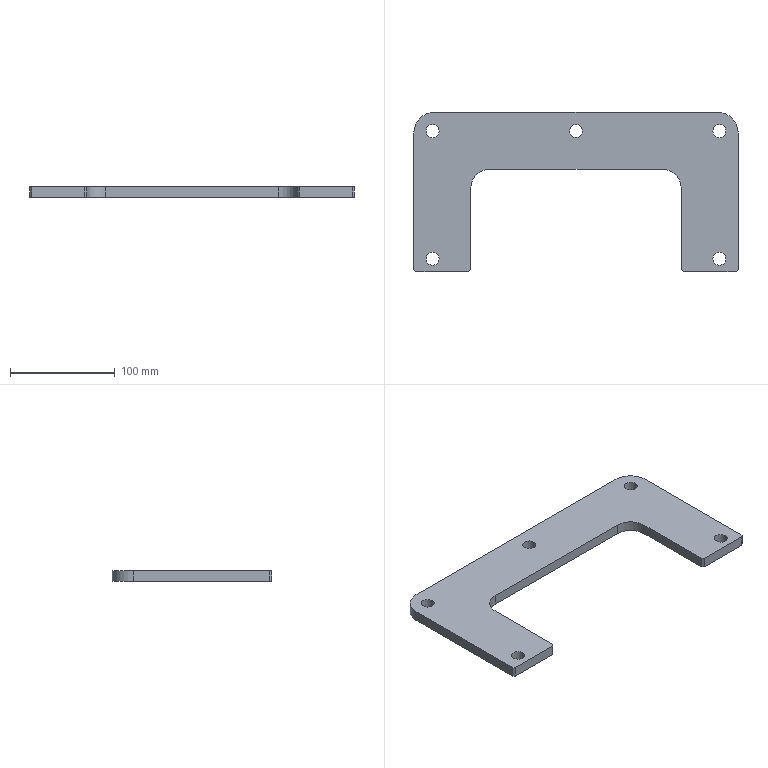Part | SolidWorks | features Chamfer 1, Extrusion 1, ICE 1 | 1 solid | 28 faces | box 310 x 152.5 x 10 mm | volume 269228 mm3 | cylinder 14 | plane 14 | commonest cylinder face diameters 12.5 x10 36 x2 40 x2
STEP:
#1=CARTESIAN_POINT('',(-143.25,15.,0.));
#2=VERTEX_POINT('',#1);
#3=CARTESIAN_POINT('',(-130.75,15.,0.));
#4=VERTEX_POINT('',#3);
#5=CARTESIAN_POINT('',(-137.,15.,0.));
#6=DIRECTION('',(0.,0.,1.));
#7=DIRECTION('',(1.,0.,0.));
#8=AXIS2_PLACEMENT_3D('',#5,#6,#7);
#9=CIRCLE('',#8,6.25);
#10=EDGE_CURVE('',#2,#4,#9,.T.);
#11=ORIENTED_EDGE('',*,*,#10,.F.);
#12=CARTESIAN_POINT('',(-143.25,15.,10.));
#13=VERTEX_POINT('',#12);
#14=CARTESIAN_POINT('',(-143.25,15.,0.));
#15=DIRECTION('',(0.,0.,1.));
#16=VECTOR('',#15,1000.);
#17=LINE('',#14,#16);
#18=EDGE_CURVE('',#2,#13,#17,.T.);
#19=ORIENTED_EDGE('',*,*,#18,.T.);
#20=CARTESIAN_POINT('',(-130.75,15.,10.));
#21=VERTEX_POINT('',#20);
#22=CARTESIAN_POINT('',(-137.,15.,10.));
#23=DIRECTION('',(0.,0.,1.));
#24=DIRECTION('',(1.,0.,0.));
#25=AXIS2_PLACEMENT_3D('',#22,#23,#24);
#26=CIRCLE('',#25,6.25);
#27=EDGE_CURVE('',#13,#21,#26,.T.);
#28=ORIENTED_EDGE('',*,*,#27,.T.);
#29=CARTESIAN_POINT('',(-130.75,15.,0.));
#30=DIRECTION('',(0.,0.,1.));
#31=VECTOR('',#30,1000.);
#32=LINE('',#29,#31);
#33=EDGE_CURVE('',#4,#21,#32,.T.);
#34=ORIENTED_EDGE('',*,*,#33,.F.);
#35=EDGE_LOOP('',(#11,#19,#28,#34));
#36=FACE_OUTER_BOUND('',#35,.T.);
#37=CARTESIAN_POINT('',(-137.,15.,0.));
#38=DIRECTION('',(0.,0.,1.));
#39=DIRECTION('',(1.,0.,0.));
#40=AXIS2_PLACEMENT_3D('',#37,#38,#39);
#41=CYLINDRICAL_SURFACE('',#40,6.25);
#42=ADVANCED_FACE('',(#36),#41,.F.);
#43=CARTESIAN_POINT('',(130.75,15.,0.));
#44=VERTEX_POINT('',#43);
#45=CARTESIAN_POINT('',(143.25,15.,0.));
#46=VERTEX_POINT('',#45);
#47=CARTESIAN_POINT('',(137.,15.,0.));
#48=DIRECTION('',(0.,0.,1.));
#49=DIRECTION('',(-1.,0.,0.));
#50=AXIS2_PLACEMENT_3D('',#47,#48,#49);
#51=CIRCLE('',#50,6.25);
#52=EDGE_CURVE('',#44,#46,#51,.T.);
#53=ORIENTED_EDGE('',*,*,#52,.F.);
#54=CARTESIAN_POINT('',(130.75,15.,10.));
#55=VERTEX_POINT('',#54);
#56=CARTESIAN_POINT('',(130.75,15.,0.));
#57=DIRECTION('',(0.,0.,1.));
#58=VECTOR('',#57,1000.);
#59=LINE('',#56,#58);
#60=EDGE_CURVE('',#44,#55,#59,.T.);
#61=ORIENTED_EDGE('',*,*,#60,.T.);
#62=CARTESIAN_POINT('',(143.25,15.,10.));
#63=VERTEX_POINT('',#62);
#64=CARTESIAN_POINT('',(137.,15.,10.));
#65=DIRECTION('',(0.,0.,1.));
#66=DIRECTION('',(-1.,0.,0.));
#67=AXIS2_PLACEMENT_3D('',#64,#65,#66);
#68=CIRCLE('',#67,6.25);
#69=EDGE_CURVE('',#55,#63,#68,.T.);
#70=ORIENTED_EDGE('',*,*,#69,.T.);
#71=CARTESIAN_POINT('',(143.25,15.,0.));
#72=DIRECTION('',(0.,0.,1.));
#73=VECTOR('',#72,1000.);
#74=LINE('',#71,#73);
#75=EDGE_CURVE('',#46,#63,#74,.T.);
#76=ORIENTED_EDGE('',*,*,#75,.F.);
#77=EDGE_LOOP('',(#53,#61,#70,#76));
#78=FACE_OUTER_BOUND('',#77,.T.);
#79=CARTESIAN_POINT('',(137.,15.,0.));
#80=DIRECTION('',(0.,0.,1.));
#81=DIRECTION('',(1.,0.,0.));
#82=AXIS2_PLACEMENT_3D('',#79,#80,#81);
#83=CYLINDRICAL_SURFACE('',#82,6.25);
#84=ADVANCED_FACE('',(#78),#83,.F.);
#85=CARTESIAN_POINT('',(-143.25,137.,0.));
#86=VERTEX_POINT('',#85);
#87=CARTESIAN_POINT('',(-130.75,137.,0.));
#88=VERTEX_POINT('',#87);
#89=CARTESIAN_POINT('',(-137.,137.,0.));
#90=DIRECTION('',(0.,0.,1.));
#91=DIRECTION('',(1.,0.,0.));
#92=AXIS2_PLACEMENT_3D('',#89,#90,#91);
#93=CIRCLE('',#92,6.25);
#94=EDGE_CURVE('',#86,#88,#93,.T.);
#95=ORIENTED_EDGE('',*,*,#94,.F.);
#96=CARTESIAN_POINT('',(-143.25,137.,10.));
#97=VERTEX_POINT('',#96);
#98=CARTESIAN_POINT('',(-143.25,137.,0.));
#99=DIRECTION('',(0.,0.,1.));
#100=VECTOR('',#99,1000.);
#101=LINE('',#98,#100);
#102=EDGE_CURVE('',#86,#97,#101,.T.);
#103=ORIENTED_EDGE('',*,*,#102,.T.);
#104=CARTESIAN_POINT('',(-130.75,137.,10.));
#105=VERTEX_POINT('',#104);
#106=CARTESIAN_POINT('',(-137.,137.,10.));
#107=DIRECTION('',(0.,0.,1.));
#108=DIRECTION('',(1.,0.,0.));
#109=AXIS2_PLACEMENT_3D('',#106,#107,#108);
#110=CIRCLE('',#109,6.25);
#111=EDGE_CURVE('',#97,#105,#110,.T.);
#112=ORIENTED_EDGE('',*,*,#111,.T.);
#113=CARTESIAN_POINT('',(-130.75,137.,0.));
#114=DIRECTION('',(0.,0.,1.));
#115=VECTOR('',#114,1000.);
#116=LINE('',#113,#115);
#117=EDGE_CURVE('',#88,#105,#116,.T.);
#118=ORIENTED_EDGE('',*,*,#117,.F.);
#119=EDGE_LOOP('',(#95,#103,#112,#118));
#120=FACE_OUTER_BOUND('',#119,.T.);
#121=CARTESIAN_POINT('',(-137.,137.,0.));
#122=DIRECTION('',(0.,0.,1.));
#123=DIRECTION('',(1.,0.,0.));
#124=AXIS2_PLACEMENT_3D('',#121,#122,#123);
#125=CYLINDRICAL_SURFACE('',#124,6.25);
#126=ADVANCED_FACE('',(#120),#125,.F.);
#127=CARTESIAN_POINT('',(130.75,137.,0.));
#128=VERTEX_POINT('',#127);
#129=CARTESIAN_POINT('',(143.25,137.,0.));
#130=VERTEX_POINT('',#129);
#131=CARTESIAN_POINT('',(137.,137.,0.));
#132=DIRECTION('',(0.,0.,1.));
#133=DIRECTION('',(1.,0.,0.));
#134=AXIS2_PLACEMENT_3D('',#131,#132,#133);
#135=CIRCLE('',#134,6.25);
#136=EDGE_CURVE('',#128,#130,#135,.T.);
#137=ORIENTED_EDGE('',*,*,#136,.F.);
#138=CARTESIAN_POINT('',(130.75,137.,10.));
#139=VERTEX_POINT('',#138);
#140=CARTESIAN_POINT('',(130.75,137.,0.));
#141=DIRECTION('',(0.,0.,1.));
#142=VECTOR('',#141,1000.);
#143=LINE('',#140,#142);
#144=EDGE_CURVE('',#128,#139,#143,.T.);
#145=ORIENTED_EDGE('',*,*,#144,.T.);
#146=CARTESIAN_POINT('',(143.25,137.,10.));
#147=VERTEX_POINT('',#146);
#148=CARTESIAN_POINT('',(137.,137.,10.));
#149=DIRECTION('',(0.,0.,1.));
#150=DIRECTION('',(1.,0.,0.));
#151=AXIS2_PLACEMENT_3D('',#148,#149,#150);
#152=CIRCLE('',#151,6.25);
#153=EDGE_CURVE('',#139,#147,#152,.T.);
#154=ORIENTED_EDGE('',*,*,#153,.T.);
#155=CARTESIAN_POINT('',(143.25,137.,0.));
#156=DIRECTION('',(0.,0.,1.));
#157=VECTOR('',#156,1000.);
#158=LINE('',#155,#157);
#159=EDGE_CURVE('',#130,#147,#158,.T.);
#160=ORIENTED_EDGE('',*,*,#159,.F.);
#161=EDGE_LOOP('',(#137,#145,#154,#160));
#162=FACE_OUTER_BOUND('',#161,.T.);
#163=CARTESIAN_POINT('',(137.,137.,0.));
#164=DIRECTION('',(0.,0.,1.));
#165=DIRECTION('',(1.,0.,0.));
#166=AXIS2_PLACEMENT_3D('',#163,#164,#165);
#167=CYLINDRICAL_SURFACE('',#166,6.25);
#168=ADVANCED_FACE('',(#162),#167,.F.);
#169=CARTESIAN_POINT('',(-6.25,137.,0.));
#170=VERTEX_POINT('',#169);
#171=CARTESIAN_POINT('',(6.25,137.,0.));
#172=VERTEX_POINT('',#171);
#173=CARTESIAN_POINT('',(0.,137.,0.));
#174=DIRECTION('',(0.,0.,1.));
#175=DIRECTION('',(1.,0.,0.));
#176=AXIS2_PLACEMENT_3D('',#173,#174,#175);
#177=CIRCLE('',#176,6.25);
#178=EDGE_CURVE('',#170,#172,#177,.T.);
#179=ORIENTED_EDGE('',*,*,#178,.F.);
#180=CARTESIAN_POINT('',(-6.25,137.,10.));
#181=VERTEX_POINT('',#180);
#182=CARTESIAN_POINT('',(-6.25,137.,0.));
#183=DIRECTION('',(0.,0.,1.));
#184=VECTOR('',#183,1000.);
#185=LINE('',#182,#184);
#186=EDGE_CURVE('',#170,#181,#185,.T.);
#187=ORIENTED_EDGE('',*,*,#186,.T.);
#188=CARTESIAN_POINT('',(6.25,137.,10.));
#189=VERTEX_POINT('',#188);
#190=CARTESIAN_POINT('',(0.,137.,10.));
#191=DIRECTION('',(0.,0.,1.));
#192=DIRECTION('',(1.,0.,0.));
#193=AXIS2_PLACEMENT_3D('',#190,#191,#192);
#194=CIRCLE('',#193,6.25);
#195=EDGE_CURVE('',#181,#189,#194,.T.);
#196=ORIENTED_EDGE('',*,*,#195,.T.);
#197=CARTESIAN_POINT('',(6.25,137.,0.));
#198=DIRECTION('',(0.,0.,1.));
#199=VECTOR('',#198,1000.);
#200=LINE('',#197,#199);
#201=EDGE_CURVE('',#172,#189,#200,.T.);
#202=ORIENTED_EDGE('',*,*,#201,.F.);
#203=EDGE_LOOP('',(#179,#187,#196,#202));
#204=FACE_OUTER_BOUND('',#203,.T.);
#205=CARTESIAN_POINT('',(0.,137.,0.));
#206=DIRECTION('',(0.,0.,1.));
#207=DIRECTION('',(1.,0.,0.));
#208=AXIS2_PLACEMENT_3D('',#205,#206,#207);
#209=CYLINDRICAL_SURFACE('',#208,6.25);
#210=ADVANCED_FACE('',(#204),#209,.F.);
#211=CARTESIAN_POINT('',(82.5,100.5,0.));
#212=VERTEX_POINT('',#211);
#213=CARTESIAN_POINT('',(100.5,82.5,0.));
#214=VERTEX_POINT('',#213);
#215=CARTESIAN_POINT('',(82.5,82.5,0.));
#216=DIRECTION('',(0.,0.,-1.));
#217=DIRECTION('',(1.,0.,0.));
#218=AXIS2_PLACEMENT_3D('',#215,#216,#217);
#219=CIRCLE('',#218,18.);
#220=EDGE_CURVE('',#212,#214,#219,.T.);
#221=ORIENTED_EDGE('',*,*,#220,.T.);
#222=CARTESIAN_POINT('',(100.5,82.5,10.));
#223=VERTEX_POINT('',#222);
#224=CARTESIAN_POINT('',(100.5,82.5,10.));
#225=DIRECTION('',(0.,0.,-1.));
#226=VECTOR('',#225,1000.);
#227=LINE('',#224,#226);
#228=EDGE_CURVE('',#223,#214,#227,.T.);
#229=ORIENTED_EDGE('',*,*,#228,.F.);
#230=CARTESIAN_POINT('',(82.5,100.5,10.));
#231=VERTEX_POINT('',#230);
#232=CARTESIAN_POINT('',(82.5,82.5,10.));
#233=DIRECTION('',(0.,0.,-1.));
#234=DIRECTION('',(1.,0.,0.));
#235=AXIS2_PLACEMENT_3D('',#232,#233,#234);
#236=CIRCLE('',#235,18.);
#237=EDGE_CURVE('',#231,#223,#236,.T.);
#238=ORIENTED_EDGE('',*,*,#237,.F.);
#239=CARTESIAN_POINT('',(82.5,100.5,10.));
#240=DIRECTION('',(0.,0.,-1.));
#241=VECTOR('',#240,1000.);
#242=LINE('',#239,#241);
#243=EDGE_CURVE('',#231,#212,#242,.T.);
#244=ORIENTED_EDGE('',*,*,#243,.T.);
#245=EDGE_LOOP('',(#221,#229,#238,#244));
#246=FACE_OUTER_BOUND('',#245,.T.);
#247=CARTESIAN_POINT('',(82.5,82.5,10.));
#248=DIRECTION('',(0.,0.,-1.));
#249=DIRECTION('',(-1.,0.,0.));
#250=AXIS2_PLACEMENT_3D('',#247,#248,#249);
#251=CYLINDRICAL_SURFACE('',#250,18.);
#252=ADVANCED_FACE('',(#246),#251,.F.);
#253=CARTESIAN_POINT('',(100.5,4.5,0.));
#254=VERTEX_POINT('',#253);
#255=CARTESIAN_POINT('',(100.5,82.5,0.));
#256=DIRECTION('',(0.,-1.,0.));
#257=VECTOR('',#256,1000.);
#258=LINE('',#255,#257);
#259=EDGE_CURVE('',#214,#254,#258,.T.);
#260=ORIENTED_EDGE('',*,*,#259,.T.);
#261=CARTESIAN_POINT('',(100.5,4.5,10.));
#262=VERTEX_POINT('',#261);
#263=CARTESIAN_POINT('',(100.5,4.5,10.));
#264=DIRECTION('',(0.,0.,1.));
#265=VECTOR('',#264,1000.);
#266=LINE('',#263,#265);
#267=EDGE_CURVE('',#254,#262,#266,.T.);
#268=ORIENTED_EDGE('',*,*,#267,.T.);
#269=CARTESIAN_POINT('',(100.5,82.5,10.));
#270=DIRECTION('',(0.,-1.,0.));
#271=VECTOR('',#270,1000.);
#272=LINE('',#269,#271);
#273=EDGE_CURVE('',#223,#262,#272,.T.);
#274=ORIENTED_EDGE('',*,*,#273,.F.);
#275=ORIENTED_EDGE('',*,*,#228,.T.);
#276=EDGE_LOOP('',(#260,#268,#274,#275));
#277=FACE_OUTER_BOUND('',#276,.T.);
#278=CARTESIAN_POINT('',(100.5,82.5,10.));
#279=DIRECTION('',(1.,0.,0.));
#280=DIRECTION('',(0.,0.,-1.));
#281=AXIS2_PLACEMENT_3D('',#278,#279,#280);
#282=PLANE('',#281);
#283=ADVANCED_FACE('',(#277),#282,.F.);
#284=CARTESIAN_POINT('',(102.5,2.5,0.));
#285=VERTEX_POINT('',#284);
#286=CARTESIAN_POINT('',(153.,2.5,0.));
#287=VERTEX_POINT('',#286);
#288=CARTESIAN_POINT('',(100.5,2.5,0.));
#289=DIRECTION('',(1.,0.,0.));
#290=VECTOR('',#289,1000.);
#291=LINE('',#288,#290);
#292=EDGE_CURVE('',#285,#287,#291,.T.);
#293=ORIENTED_EDGE('',*,*,#292,.T.);
#294=CARTESIAN_POINT('',(153.,2.5,10.));
#295=VERTEX_POINT('',#294);
#296=CARTESIAN_POINT('',(153.,2.5,10.));
#297=DIRECTION('',(0.,0.,1.));
#298=VECTOR('',#297,1000.);
#299=LINE('',#296,#298);
#300=EDGE_CURVE('',#287,#295,#299,.T.);
#301=ORIENTED_EDGE('',*,*,#300,.T.);
#302=CARTESIAN_POINT('',(102.5,2.5,10.));
#303=VERTEX_POINT('',#302);
#304=CARTESIAN_POINT('',(100.5,2.5,10.));
#305=DIRECTION('',(1.,0.,0.));
#306=VECTOR('',#305,1000.);
#307=LINE('',#304,#306);
#308=EDGE_CURVE('',#303,#295,#307,.T.);
#309=ORIENTED_EDGE('',*,*,#308,.F.);
#310=CARTESIAN_POINT('',(102.5,2.5,10.));
#311=DIRECTION('',(0.,0.,-1.));
#312=VECTOR('',#311,1000.);
#313=LINE('',#310,#312);
#314=EDGE_CURVE('',#303,#285,#313,.T.);
#315=ORIENTED_EDGE('',*,*,#314,.T.);
#316=EDGE_LOOP('',(#293,#301,#309,#315));
#317=FACE_OUTER_BOUND('',#316,.T.);
#318=CARTESIAN_POINT('',(100.5,2.5,10.));
#319=DIRECTION('',(0.,1.,0.));
#320=DIRECTION('',(0.,0.,1.));
#321=AXIS2_PLACEMENT_3D('',#318,#319,#320);
#322=PLANE('',#321);
#323=ADVANCED_FACE('',(#317),#322,.F.);
#324=CARTESIAN_POINT('',(155.,4.5,10.));
#325=VERTEX_POINT('',#324);
#326=CARTESIAN_POINT('',(155.,135.,10.));
#327=VERTEX_POINT('',#326);
#328=CARTESIAN_POINT('',(155.,2.5,10.));
#329=DIRECTION('',(0.,1.,0.));
#330=VECTOR('',#329,1000.);
#331=LINE('',#328,#330);
#332=EDGE_CURVE('',#325,#327,#331,.T.);
#333=ORIENTED_EDGE('',*,*,#332,.F.);
#334=CARTESIAN_POINT('',(155.,4.5,0.));
#335=VERTEX_POINT('',#334);
#336=CARTESIAN_POINT('',(155.,4.5,10.));
#337=DIRECTION('',(0.,0.,-1.));
#338=VECTOR('',#337,1000.);
#339=LINE('',#336,#338);
#340=EDGE_CURVE('',#325,#335,#339,.T.);
#341=ORIENTED_EDGE('',*,*,#340,.T.);
#342=CARTESIAN_POINT('',(155.,135.,0.));
#343=VERTEX_POINT('',#342);
#344=CARTESIAN_POINT('',(155.,2.5,0.));
#345=DIRECTION('',(0.,1.,0.));
#346=VECTOR('',#345,1000.);
#347=LINE('',#344,#346);
#348=EDGE_CURVE('',#335,#343,#347,.T.);
#349=ORIENTED_EDGE('',*,*,#348,.T.);
#350=CARTESIAN_POINT('',(155.,135.,10.));
#351=DIRECTION('',(0.,0.,-1.));
#352=VECTOR('',#351,1000.);
#353=LINE('',#350,#352);
#354=EDGE_CURVE('',#327,#343,#353,.T.);
#355=ORIENTED_EDGE('',*,*,#354,.F.);
#356=EDGE_LOOP('',(#333,#341,#349,#355));
#357=FACE_OUTER_BOUND('',#356,.T.);
#358=CARTESIAN_POINT('',(155.,2.5,10.));
#359=DIRECTION('',(-1.,0.,0.));
#360=DIRECTION('',(0.,0.,1.));
#361=AXIS2_PLACEMENT_3D('',#358,#359,#360);
#362=PLANE('',#361);
#363=ADVANCED_FACE('',(#357),#362,.F.);
#364=CARTESIAN_POINT('',(135.,155.,0.));
#365=VERTEX_POINT('',#364);
#366=CARTESIAN_POINT('',(135.,135.,0.));
#367=DIRECTION('',(0.,0.,1.));
#368=DIRECTION('',(1.,0.,0.));
#369=AXIS2_PLACEMENT_3D('',#366,#367,#368);
#370=CIRCLE('',#369,20.);
#371=EDGE_CURVE('',#343,#365,#370,.T.);
#372=ORIENTED_EDGE('',*,*,#371,.T.);
#373=CARTESIAN_POINT('',(135.,155.,10.));
#374=VERTEX_POINT('',#373);
#375=CARTESIAN_POINT('',(135.,155.,10.));
#376=DIRECTION('',(0.,0.,-1.));
#377=VECTOR('',#376,1000.);
#378=LINE('',#375,#377);
#379=EDGE_CURVE('',#374,#365,#378,.T.);
#380=ORIENTED_EDGE('',*,*,#379,.F.);
#381=CARTESIAN_POINT('',(135.,135.,10.));
#382=DIRECTION('',(0.,0.,1.));
#383=DIRECTION('',(1.,0.,0.));
#384=AXIS2_PLACEMENT_3D('',#381,#382,#383);
#385=CIRCLE('',#384,20.);
#386=EDGE_CURVE('',#327,#374,#385,.T.);
#387=ORIENTED_EDGE('',*,*,#386,.F.);
#388=ORIENTED_EDGE('',*,*,#354,.T.);
#389=EDGE_LOOP('',(#372,#380,#387,#388));
#390=FACE_OUTER_BOUND('',#389,.T.);
#391=CARTESIAN_POINT('',(135.,135.,10.));
#392=DIRECTION('',(0.,0.,-1.));
#393=DIRECTION('',(-1.,0.,0.));
#394=AXIS2_PLACEMENT_3D('',#391,#392,#393);
#395=CYLINDRICAL_SURFACE('',#394,20.);
#396=ADVANCED_FACE('',(#390),#395,.T.);
#397=CARTESIAN_POINT('',(-135.,155.,0.));
#398=VERTEX_POINT('',#397);
#399=CARTESIAN_POINT('',(-135.,155.,0.));
#400=DIRECTION('',(-1.,0.,0.));
#401=VECTOR('',#400,1000.);
#402=LINE('',#399,#401);
#403=EDGE_CURVE('',#365,#398,#402,.T.);
#404=ORIENTED_EDGE('',*,*,#403,.T.);
#405=CARTESIAN_POINT('',(-135.,155.,10.));
#406=VERTEX_POINT('',#405);
#407=CARTESIAN_POINT('',(-135.,155.,10.));
#408=DIRECTION('',(0.,0.,-1.));
#409=VECTOR('',#408,1000.);
#410=LINE('',#407,#409);
#411=EDGE_CURVE('',#406,#398,#410,.T.);
#412=ORIENTED_EDGE('',*,*,#411,.F.);
#413=CARTESIAN_POINT('',(-135.,155.,10.));
#414=DIRECTION('',(-1.,0.,0.));
#415=VECTOR('',#414,1000.);
#416=LINE('',#413,#415);
#417=EDGE_CURVE('',#374,#406,#416,.T.);
#418=ORIENTED_EDGE('',*,*,#417,.F.);
#419=ORIENTED_EDGE('',*,*,#379,.T.);
#420=EDGE_LOOP('',(#404,#412,#418,#419));
#421=FACE_OUTER_BOUND('',#420,.T.);
#422=CARTESIAN_POINT('',(-135.,155.,10.));
#423=DIRECTION('',(0.,-1.,0.));
#424=DIRECTION('',(0.,0.,-1.));
#425=AXIS2_PLACEMENT_3D('',#422,#423,#424);
#426=PLANE('',#425);
#427=ADVANCED_FACE('',(#421),#426,.F.);
#428=CARTESIAN_POINT('',(-155.,135.,0.));
#429=VERTEX_POINT('',#428);
#430=CARTESIAN_POINT('',(-135.,135.,0.));
#431=DIRECTION('',(0.,0.,1.));
#432=DIRECTION('',(-1.,0.,0.));
#433=AXIS2_PLACEMENT_3D('',#430,#431,#432);
#434=CIRCLE('',#433,20.);
#435=EDGE_CURVE('',#398,#429,#434,.T.);
#436=ORIENTED_EDGE('',*,*,#435,.T.);
#437=CARTESIAN_POINT('',(-155.,135.,10.));
#438=VERTEX_POINT('',#437);
#439=CARTESIAN_POINT('',(-155.,135.,10.));
#440=DIRECTION('',(0.,0.,-1.));
#441=VECTOR('',#440,1000.);
#442=LINE('',#439,#441);
#443=EDGE_CURVE('',#438,#429,#442,.T.);
#444=ORIENTED_EDGE('',*,*,#443,.F.);
#445=CARTESIAN_POINT('',(-135.,135.,10.));
#446=DIRECTION('',(0.,0.,1.));
#447=DIRECTION('',(-1.,0.,0.));
#448=AXIS2_PLACEMENT_3D('',#445,#446,#447);
#449=CIRCLE('',#448,20.);
#450=EDGE_CURVE('',#406,#438,#449,.T.);
#451=ORIENTED_EDGE('',*,*,#450,.F.);
#452=ORIENTED_EDGE('',*,*,#411,.T.);
#453=EDGE_LOOP('',(#436,#444,#451,#452));
#454=FACE_OUTER_BOUND('',#453,.T.);
#455=CARTESIAN_POINT('',(-135.,135.,10.));
#456=DIRECTION('',(0.,0.,-1.));
#457=DIRECTION('',(-1.,0.,0.));
#458=AXIS2_PLACEMENT_3D('',#455,#456,#457);
#459=CYLINDRICAL_SURFACE('',#458,20.);
#460=ADVANCED_FACE('',(#454),#459,.T.);
#461=CARTESIAN_POINT('',(-155.,4.5,0.));
#462=VERTEX_POINT('',#461);
#463=CARTESIAN_POINT('',(-155.,2.5,0.));
#464=DIRECTION('',(0.,-1.,0.));
#465=VECTOR('',#464,1000.);
#466=LINE('',#463,#465);
#467=EDGE_CURVE('',#429,#462,#466,.T.);
#468=ORIENTED_EDGE('',*,*,#467,.T.);
#469=CARTESIAN_POINT('',(-155.,4.5,10.));
#470=VERTEX_POINT('',#469);
#471=CARTESIAN_POINT('',(-155.,4.5,10.));
#472=DIRECTION('',(0.,0.,1.));
#473=VECTOR('',#472,1000.);
#474=LINE('',#471,#473);
#475=EDGE_CURVE('',#462,#470,#474,.T.);
#476=ORIENTED_EDGE('',*,*,#475,.T.);
#477=CARTESIAN_POINT('',(-155.,2.5,10.));
#478=DIRECTION('',(0.,-1.,0.));
#479=VECTOR('',#478,1000.);
#480=LINE('',#477,#479);
#481=EDGE_CURVE('',#438,#470,#480,.T.);
#482=ORIENTED_EDGE('',*,*,#481,.F.);
#483=ORIENTED_EDGE('',*,*,#443,.T.);
#484=EDGE_LOOP('',(#468,#476,#482,#483));
#485=FACE_OUTER_BOUND('',#484,.T.);
#486=CARTESIAN_POINT('',(-155.,2.5,10.));
#487=DIRECTION('',(1.,0.,0.));
#488=DIRECTION('',(0.,0.,-1.));
#489=AXIS2_PLACEMENT_3D('',#486,#487,#488);
#490=PLANE('',#489);
#491=ADVANCED_FACE('',(#485),#490,.F.);
#492=CARTESIAN_POINT('',(-153.,2.5,10.));
#493=VERTEX_POINT('',#492);
#494=CARTESIAN_POINT('',(-102.5,2.5,10.));
#495=VERTEX_POINT('',#494);
#496=CARTESIAN_POINT('',(-100.5,2.5,10.));
#497=DIRECTION('',(1.,0.,0.));
#498=VECTOR('',#497,1000.);
#499=LINE('',#496,#498);
#500=EDGE_CURVE('',#493,#495,#499,.T.);
#501=ORIENTED_EDGE('',*,*,#500,.F.);
#502=CARTESIAN_POINT('',(-153.,2.5,0.));
#503=VERTEX_POINT('',#502);
#504=CARTESIAN_POINT('',(-153.,2.5,10.));
#505=DIRECTION('',(0.,0.,-1.));
#506=VECTOR('',#505,1000.);
#507=LINE('',#504,#506);
#508=EDGE_CURVE('',#493,#503,#507,.T.);
#509=ORIENTED_EDGE('',*,*,#508,.T.);
#510=CARTESIAN_POINT('',(-102.5,2.5,0.));
#511=VERTEX_POINT('',#510);
#512=CARTESIAN_POINT('',(-100.5,2.5,0.));
#513=DIRECTION('',(1.,0.,0.));
#514=VECTOR('',#513,1000.);
#515=LINE('',#512,#514);
#516=EDGE_CURVE('',#503,#511,#515,.T.);
#517=ORIENTED_EDGE('',*,*,#516,.T.);
#518=CARTESIAN_POINT('',(-102.5,2.5,10.));
#519=DIRECTION('',(0.,0.,1.));
#520=VECTOR('',#519,1000.);
#521=LINE('',#518,#520);
#522=EDGE_CURVE('',#511,#495,#521,.T.);
#523=ORIENTED_EDGE('',*,*,#522,.T.);
#524=EDGE_LOOP('',(#501,#509,#517,#523));
#525=FACE_OUTER_BOUND('',#524,.T.);
#526=CARTESIAN_POINT('',(-100.5,2.5,10.));
#527=DIRECTION('',(0.,1.,0.));
#528=DIRECTION('',(-1.,0.,0.));
#529=AXIS2_PLACEMENT_3D('',#526,#527,#528);
#530=PLANE('',#529);
#531=ADVANCED_FACE('',(#525),#530,.F.);
#532=CARTESIAN_POINT('',(-100.5,4.5,10.));
#533=VERTEX_POINT('',#532);
#534=CARTESIAN_POINT('',(-100.5,82.5,10.));
#535=VERTEX_POINT('',#534);
#536=CARTESIAN_POINT('',(-100.5,82.5,10.));
#537=DIRECTION('',(0.,1.,0.));
#538=VECTOR('',#537,1000.);
#539=LINE('',#536,#538);
#540=EDGE_CURVE('',#533,#535,#539,.T.);
#541=ORIENTED_EDGE('',*,*,#540,.F.);
#542=CARTESIAN_POINT('',(-100.5,4.5,0.));
#543=VERTEX_POINT('',#542);
#544=CARTESIAN_POINT('',(-100.5,4.5,10.));
#545=DIRECTION('',(0.,0.,-1.));
#546=VECTOR('',#545,1000.);
#547=LINE('',#544,#546);
#548=EDGE_CURVE('',#533,#543,#547,.T.);
#549=ORIENTED_EDGE('',*,*,#548,.T.);
#550=CARTESIAN_POINT('',(-100.5,82.5,0.));
#551=VERTEX_POINT('',#550);
#552=CARTESIAN_POINT('',(-100.5,82.5,0.));
#553=DIRECTION('',(0.,1.,0.));
#554=VECTOR('',#553,1000.);
#555=LINE('',#552,#554);
#556=EDGE_CURVE('',#543,#551,#555,.T.);
#557=ORIENTED_EDGE('',*,*,#556,.T.);
#558=CARTESIAN_POINT('',(-100.5,82.5,10.));
#559=DIRECTION('',(0.,0.,-1.));
#560=VECTOR('',#559,1000.);
#561=LINE('',#558,#560);
#562=EDGE_CURVE('',#535,#551,#561,.T.);
#563=ORIENTED_EDGE('',*,*,#562,.F.);
#564=EDGE_LOOP('',(#541,#549,#557,#563));
#565=FACE_OUTER_BOUND('',#564,.T.);
#566=CARTESIAN_POINT('',(-100.5,82.5,10.));
#567=DIRECTION('',(-1.,0.,0.));
#568=DIRECTION('',(0.,0.,1.));
#569=AXIS2_PLACEMENT_3D('',#566,#567,#568);
#570=PLANE('',#569);
#571=ADVANCED_FACE('',(#565),#570,.F.);
#572=CARTESIAN_POINT('',(-82.5,100.5,0.));
#573=VERTEX_POINT('',#572);
#574=CARTESIAN_POINT('',(-82.5,82.5,0.));
#575=DIRECTION('',(0.,0.,-1.));
#576=DIRECTION('',(-1.,0.,0.));
#577=AXIS2_PLACEMENT_3D('',#574,#575,#576);
#578=CIRCLE('',#577,18.);
#579=EDGE_CURVE('',#551,#573,#578,.T.);
#580=ORIENTED_EDGE('',*,*,#579,.T.);
#581=CARTESIAN_POINT('',(-82.5,100.5,10.));
#582=VERTEX_POINT('',#581);
#583=CARTESIAN_POINT('',(-82.5,100.5,10.));
#584=DIRECTION('',(0.,0.,-1.));
#585=VECTOR('',#584,1000.);
#586=LINE('',#583,#585);
#587=EDGE_CURVE('',#582,#573,#586,.T.);
#588=ORIENTED_EDGE('',*,*,#587,.F.);
#589=CARTESIAN_POINT('',(-82.5,82.5,10.));
#590=DIRECTION('',(0.,0.,-1.));
#591=DIRECTION('',(-1.,0.,0.));
#592=AXIS2_PLACEMENT_3D('',#589,#590,#591);
#593=CIRCLE('',#592,18.);
#594=EDGE_CURVE('',#535,#582,#593,.T.);
#595=ORIENTED_EDGE('',*,*,#594,.F.);
#596=ORIENTED_EDGE('',*,*,#562,.T.);
#597=EDGE_LOOP('',(#580,#588,#595,#596));
#598=FACE_OUTER_BOUND('',#597,.T.);
#599=CARTESIAN_POINT('',(-82.5,82.5,10.));
#600=DIRECTION('',(0.,0.,-1.));
#601=DIRECTION('',(-1.,0.,0.));
#602=AXIS2_PLACEMENT_3D('',#599,#600,#601);
#603=CYLINDRICAL_SURFACE('',#602,18.);
#604=ADVANCED_FACE('',(#598),#603,.F.);
#605=CARTESIAN_POINT('',(-82.5,100.5,0.));
#606=DIRECTION('',(1.,0.,0.));
#607=VECTOR('',#606,1000.);
#608=LINE('',#605,#607);
#609=EDGE_CURVE('',#573,#212,#608,.T.);
#610=ORIENTED_EDGE('',*,*,#609,.T.);
#611=ORIENTED_EDGE('',*,*,#243,.F.);
#612=CARTESIAN_POINT('',(-82.5,100.5,10.));
#613=DIRECTION('',(1.,0.,0.));
#614=VECTOR('',#613,1000.);
#615=LINE('',#612,#614);
#616=EDGE_CURVE('',#582,#231,#615,.T.);
#617=ORIENTED_EDGE('',*,*,#616,.F.);
#618=ORIENTED_EDGE('',*,*,#587,.T.);
#619=EDGE_LOOP('',(#610,#611,#617,#618));
#620=FACE_OUTER_BOUND('',#619,.T.);
#621=CARTESIAN_POINT('',(-82.5,100.5,10.));
#622=DIRECTION('',(0.,1.,0.));
#623=DIRECTION('',(0.,0.,1.));
#624=AXIS2_PLACEMENT_3D('',#621,#622,#623);
#625=PLANE('',#624);
#626=ADVANCED_FACE('',(#620),#625,.F.);
#627=CARTESIAN_POINT('',(-137.,15.,10.));
#628=DIRECTION('',(0.,0.,1.));
#629=DIRECTION('',(1.,0.,0.));
#630=AXIS2_PLACEMENT_3D('',#627,#628,#629);
#631=CIRCLE('',#630,6.25);
#632=EDGE_CURVE('',#21,#13,#631,.T.);
#633=ORIENTED_EDGE('',*,*,#632,.F.);
#634=ORIENTED_EDGE('',*,*,#27,.F.);
#635=EDGE_LOOP('',(#633,#634));
#636=FACE_BOUND('',#635,.T.);
#637=CARTESIAN_POINT('',(137.,15.,10.));
#638=DIRECTION('',(0.,0.,1.));
#639=DIRECTION('',(-1.,0.,0.));
#640=AXIS2_PLACEMENT_3D('',#637,#638,#639);
#641=CIRCLE('',#640,6.25);
#642=EDGE_CURVE('',#63,#55,#641,.T.);
#643=ORIENTED_EDGE('',*,*,#642,.F.);
#644=ORIENTED_EDGE('',*,*,#69,.F.);
#645=EDGE_LOOP('',(#643,#644));
#646=FACE_BOUND('',#645,.T.);
#647=CARTESIAN_POINT('',(-137.,137.,10.));
#648=DIRECTION('',(0.,0.,1.));
#649=DIRECTION('',(1.,0.,0.));
#650=AXIS2_PLACEMENT_3D('',#647,#648,#649);
#651=CIRCLE('',#650,6.25);
#652=EDGE_CURVE('',#105,#97,#651,.T.);
#653=ORIENTED_EDGE('',*,*,#652,.F.);
#654=ORIENTED_EDGE('',*,*,#111,.F.);
#655=EDGE_LOOP('',(#653,#654));
#656=FACE_BOUND('',#655,.T.);
#657=CARTESIAN_POINT('',(137.,137.,10.));
#658=DIRECTION('',(0.,0.,1.));
#659=DIRECTION('',(1.,0.,0.));
#660=AXIS2_PLACEMENT_3D('',#657,#658,#659);
#661=CIRCLE('',#660,6.25);
#662=EDGE_CURVE('',#147,#139,#661,.T.);
#663=ORIENTED_EDGE('',*,*,#662,.F.);
#664=ORIENTED_EDGE('',*,*,#153,.F.);
#665=EDGE_LOOP('',(#663,#664));
#666=FACE_BOUND('',#665,.T.);
#667=CARTESIAN_POINT('',(0.,137.,10.));
#668=DIRECTION('',(0.,0.,1.));
#669=DIRECTION('',(1.,0.,0.));
#670=AXIS2_PLACEMENT_3D('',#667,#668,#669);
#671=CIRCLE('',#670,6.25);
#672=EDGE_CURVE('',#189,#181,#671,.T.);
#673=ORIENTED_EDGE('',*,*,#672,.F.);
#674=ORIENTED_EDGE('',*,*,#195,.F.);
#675=EDGE_LOOP('',(#673,#674));
#676=FACE_BOUND('',#675,.T.);
#677=ORIENTED_EDGE('',*,*,#308,.T.);
#678=CARTESIAN_POINT('',(157.75,7.25,10.));
#679=DIRECTION('',(0.7071,0.7071,0.));
#680=VECTOR('',#679,1000.);
#681=LINE('',#678,#680);
#682=EDGE_CURVE('',#295,#325,#681,.T.);
#683=ORIENTED_EDGE('',*,*,#682,.T.);
#684=ORIENTED_EDGE('',*,*,#332,.T.);
#685=ORIENTED_EDGE('',*,*,#386,.T.);
#686=ORIENTED_EDGE('',*,*,#417,.T.);
#687=ORIENTED_EDGE('',*,*,#450,.T.);
#688=ORIENTED_EDGE('',*,*,#481,.T.);
#689=CARTESIAN_POINT('',(-75.25,-75.25,10.));
#690=DIRECTION('',(0.7071,-0.7071,0.));
#691=VECTOR('',#690,1000.);
#692=LINE('',#689,#691);
#693=EDGE_CURVE('',#470,#493,#692,.T.);
#694=ORIENTED_EDGE('',*,*,#693,.T.);
#695=ORIENTED_EDGE('',*,*,#500,.T.);
#696=CARTESIAN_POINT('',(30.,135.,10.));
#697=DIRECTION('',(0.7071,0.7071,0.));
#698=VECTOR('',#697,1000.);
#699=LINE('',#696,#698);
#700=EDGE_CURVE('',#495,#533,#699,.T.);
#701=ORIENTED_EDGE('',*,*,#700,.T.);
#702=ORIENTED_EDGE('',*,*,#540,.T.);
#703=ORIENTED_EDGE('',*,*,#594,.T.);
#704=ORIENTED_EDGE('',*,*,#616,.T.);
#705=ORIENTED_EDGE('',*,*,#237,.T.);
#706=ORIENTED_EDGE('',*,*,#273,.T.);
#707=CARTESIAN_POINT('',(52.5,52.5,10.));
#708=DIRECTION('',(0.7071,-0.7071,0.));
#709=VECTOR('',#708,1000.);
#710=LINE('',#707,#709);
#711=EDGE_CURVE('',#262,#303,#710,.T.);
#712=ORIENTED_EDGE('',*,*,#711,.T.);
#713=EDGE_LOOP('',(#677,#683,#684,#685,#686,#687,#688,#694,#695,#701,#702,#703,#704,#705,#706,#712));
#714=FACE_OUTER_BOUND('',#713,.T.);
#715=CARTESIAN_POINT('',(82.5,82.5,10.));
#716=DIRECTION('',(0.,0.,1.));
#717=DIRECTION('',(1.,0.,0.));
#718=AXIS2_PLACEMENT_3D('',#715,#716,#717);
#719=PLANE('',#718);
#720=ADVANCED_FACE('',(#636,#646,#656,#666,#676,#714),#719,.T.);
#721=CARTESIAN_POINT('',(-137.,15.,0.));
#722=DIRECTION('',(0.,0.,1.));
#723=DIRECTION('',(1.,0.,0.));
#724=AXIS2_PLACEMENT_3D('',#721,#722,#723);
#725=CIRCLE('',#724,6.25);
#726=EDGE_CURVE('',#4,#2,#725,.T.);
#727=ORIENTED_EDGE('',*,*,#726,.T.);
#728=ORIENTED_EDGE('',*,*,#10,.T.);
#729=EDGE_LOOP('',(#727,#728));
#730=FACE_BOUND('',#729,.T.);
#731=CARTESIAN_POINT('',(137.,15.,0.));
#732=DIRECTION('',(0.,0.,1.));
#733=DIRECTION('',(-1.,0.,0.));
#734=AXIS2_PLACEMENT_3D('',#731,#732,#733);
#735=CIRCLE('',#734,6.25);
#736=EDGE_CURVE('',#46,#44,#735,.T.);
#737=ORIENTED_EDGE('',*,*,#736,.T.);
#738=ORIENTED_EDGE('',*,*,#52,.T.);
#739=EDGE_LOOP('',(#737,#738));
#740=FACE_BOUND('',#739,.T.);
#741=CARTESIAN_POINT('',(-137.,137.,0.));
#742=DIRECTION('',(0.,0.,1.));
#743=DIRECTION('',(1.,0.,0.));
#744=AXIS2_PLACEMENT_3D('',#741,#742,#743);
#745=CIRCLE('',#744,6.25);
#746=EDGE_CURVE('',#88,#86,#745,.T.);
#747=ORIENTED_EDGE('',*,*,#746,.T.);
#748=ORIENTED_EDGE('',*,*,#94,.T.);
#749=EDGE_LOOP('',(#747,#748));
#750=FACE_BOUND('',#749,.T.);
#751=CARTESIAN_POINT('',(137.,137.,0.));
#752=DIRECTION('',(0.,0.,1.));
#753=DIRECTION('',(1.,0.,0.));
#754=AXIS2_PLACEMENT_3D('',#751,#752,#753);
#755=CIRCLE('',#754,6.25);
#756=EDGE_CURVE('',#130,#128,#755,.T.);
#757=ORIENTED_EDGE('',*,*,#756,.T.);
#758=ORIENTED_EDGE('',*,*,#136,.T.);
#759=EDGE_LOOP('',(#757,#758));
#760=FACE_BOUND('',#759,.T.);
#761=CARTESIAN_POINT('',(0.,137.,0.));
#762=DIRECTION('',(0.,0.,1.));
#763=DIRECTION('',(1.,0.,0.));
#764=AXIS2_PLACEMENT_3D('',#761,#762,#763);
#765=CIRCLE('',#764,6.25);
#766=EDGE_CURVE('',#172,#170,#765,.T.);
#767=ORIENTED_EDGE('',*,*,#766,.T.);
#768=ORIENTED_EDGE('',*,*,#178,.T.);
#769=EDGE_LOOP('',(#767,#768));
#770=FACE_BOUND('',#769,.T.);
#771=ORIENTED_EDGE('',*,*,#348,.F.);
#772=CARTESIAN_POINT('',(155.,4.5,0.));
#773=DIRECTION('',(-0.7071,-0.7071,0.));
#774=VECTOR('',#773,1000.);
#775=LINE('',#772,#774);
#776=EDGE_CURVE('',#335,#287,#775,.T.);
#777=ORIENTED_EDGE('',*,*,#776,.T.);
#778=ORIENTED_EDGE('',*,*,#292,.F.);
#779=CARTESIAN_POINT('',(102.5,2.5,0.));
#780=DIRECTION('',(-0.7071,0.7071,0.));
#781=VECTOR('',#780,1000.);
#782=LINE('',#779,#781);
#783=EDGE_CURVE('',#285,#254,#782,.T.);
#784=ORIENTED_EDGE('',*,*,#783,.T.);
#785=ORIENTED_EDGE('',*,*,#259,.F.);
#786=ORIENTED_EDGE('',*,*,#220,.F.);
#787=ORIENTED_EDGE('',*,*,#609,.F.);
#788=ORIENTED_EDGE('',*,*,#579,.F.);
#789=ORIENTED_EDGE('',*,*,#556,.F.);
#790=CARTESIAN_POINT('',(-100.5,4.5,0.));
#791=DIRECTION('',(-0.7071,-0.7071,0.));
#792=VECTOR('',#791,1000.);
#793=LINE('',#790,#792);
#794=EDGE_CURVE('',#543,#511,#793,.T.);
#795=ORIENTED_EDGE('',*,*,#794,.T.);
#796=ORIENTED_EDGE('',*,*,#516,.F.);
#797=CARTESIAN_POINT('',(-153.,2.5,0.));
#798=DIRECTION('',(-0.7071,0.7071,0.));
#799=VECTOR('',#798,1000.);
#800=LINE('',#797,#799);
#801=EDGE_CURVE('',#503,#462,#800,.T.);
#802=ORIENTED_EDGE('',*,*,#801,.T.);
#803=ORIENTED_EDGE('',*,*,#467,.F.);
#804=ORIENTED_EDGE('',*,*,#435,.F.);
#805=ORIENTED_EDGE('',*,*,#403,.F.);
#806=ORIENTED_EDGE('',*,*,#371,.F.);
#807=EDGE_LOOP('',(#771,#777,#778,#784,#785,#786,#787,#788,#789,#795,#796,#802,#803,#804,#805,#806));
#808=FACE_OUTER_BOUND('',#807,.T.);
#809=CARTESIAN_POINT('',(82.5,82.5,0.));
#810=DIRECTION('',(0.,0.,1.));
#811=DIRECTION('',(1.,0.,0.));
#812=AXIS2_PLACEMENT_3D('',#809,#810,#811);
#813=PLANE('',#812);
#814=ADVANCED_FACE('',(#730,#740,#750,#760,#770,#808),#813,.F.);
#815=ORIENTED_EDGE('',*,*,#186,.F.);
#816=ORIENTED_EDGE('',*,*,#766,.F.);
#817=ORIENTED_EDGE('',*,*,#201,.T.);
#818=ORIENTED_EDGE('',*,*,#672,.T.);
#819=EDGE_LOOP('',(#815,#816,#817,#818));
#820=FACE_OUTER_BOUND('',#819,.T.);
#821=CARTESIAN_POINT('',(0.,137.,0.));
#822=DIRECTION('',(0.,0.,1.));
#823=DIRECTION('',(1.,0.,0.));
#824=AXIS2_PLACEMENT_3D('',#821,#822,#823);
#825=CYLINDRICAL_SURFACE('',#824,6.25);
#826=ADVANCED_FACE('',(#820),#825,.F.);
#827=ORIENTED_EDGE('',*,*,#144,.F.);
#828=ORIENTED_EDGE('',*,*,#756,.F.);
#829=ORIENTED_EDGE('',*,*,#159,.T.);
#830=ORIENTED_EDGE('',*,*,#662,.T.);
#831=EDGE_LOOP('',(#827,#828,#829,#830));
#832=FACE_OUTER_BOUND('',#831,.T.);
#833=CARTESIAN_POINT('',(137.,137.,0.));
#834=DIRECTION('',(0.,0.,1.));
#835=DIRECTION('',(1.,0.,0.));
#836=AXIS2_PLACEMENT_3D('',#833,#834,#835);
#837=CYLINDRICAL_SURFACE('',#836,6.25);
#838=ADVANCED_FACE('',(#832),#837,.F.);
#839=ORIENTED_EDGE('',*,*,#102,.F.);
#840=ORIENTED_EDGE('',*,*,#746,.F.);
#841=ORIENTED_EDGE('',*,*,#117,.T.);
#842=ORIENTED_EDGE('',*,*,#652,.T.);
#843=EDGE_LOOP('',(#839,#840,#841,#842));
#844=FACE_OUTER_BOUND('',#843,.T.);
#845=CARTESIAN_POINT('',(-137.,137.,0.));
#846=DIRECTION('',(0.,0.,1.));
#847=DIRECTION('',(1.,0.,0.));
#848=AXIS2_PLACEMENT_3D('',#845,#846,#847);
#849=CYLINDRICAL_SURFACE('',#848,6.25);
#850=ADVANCED_FACE('',(#844),#849,.F.);
#851=ORIENTED_EDGE('',*,*,#60,.F.);
#852=ORIENTED_EDGE('',*,*,#736,.F.);
#853=ORIENTED_EDGE('',*,*,#75,.T.);
#854=ORIENTED_EDGE('',*,*,#642,.T.);
#855=EDGE_LOOP('',(#851,#852,#853,#854));
#856=FACE_OUTER_BOUND('',#855,.T.);
#857=CARTESIAN_POINT('',(137.,15.,0.));
#858=DIRECTION('',(0.,0.,1.));
#859=DIRECTION('',(1.,0.,0.));
#860=AXIS2_PLACEMENT_3D('',#857,#858,#859);
#861=CYLINDRICAL_SURFACE('',#860,6.25);
#862=ADVANCED_FACE('',(#856),#861,.F.);
#863=ORIENTED_EDGE('',*,*,#18,.F.);
#864=ORIENTED_EDGE('',*,*,#726,.F.);
#865=ORIENTED_EDGE('',*,*,#33,.T.);
#866=ORIENTED_EDGE('',*,*,#632,.T.);
#867=EDGE_LOOP('',(#863,#864,#865,#866));
#868=FACE_OUTER_BOUND('',#867,.T.);
#869=CARTESIAN_POINT('',(-137.,15.,0.));
#870=DIRECTION('',(0.,0.,1.));
#871=DIRECTION('',(1.,0.,0.));
#872=AXIS2_PLACEMENT_3D('',#869,#870,#871);
#873=CYLINDRICAL_SURFACE('',#872,6.25);
#874=ADVANCED_FACE('',(#868),#873,.F.);
#875=ORIENTED_EDGE('',*,*,#682,.F.);
#876=ORIENTED_EDGE('',*,*,#300,.F.);
#877=ORIENTED_EDGE('',*,*,#776,.F.);
#878=ORIENTED_EDGE('',*,*,#340,.F.);
#879=EDGE_LOOP('',(#875,#876,#877,#878));
#880=FACE_OUTER_BOUND('',#879,.T.);
#881=CARTESIAN_POINT('',(155.,4.5,10.));
#882=DIRECTION('',(-0.7071,0.7071,0.));
#883=DIRECTION('',(0.,0.,-1.));
#884=AXIS2_PLACEMENT_3D('',#881,#882,#883);
#885=PLANE('',#884);
#886=ADVANCED_FACE('',(#880),#885,.F.);
#887=ORIENTED_EDGE('',*,*,#711,.F.);
#888=ORIENTED_EDGE('',*,*,#267,.F.);
#889=ORIENTED_EDGE('',*,*,#783,.F.);
#890=ORIENTED_EDGE('',*,*,#314,.F.);
#891=EDGE_LOOP('',(#887,#888,#889,#890));
#892=FACE_OUTER_BOUND('',#891,.T.);
#893=CARTESIAN_POINT('',(102.5,2.5,10.));
#894=DIRECTION('',(0.7071,0.7071,0.));
#895=DIRECTION('',(0.,0.,-1.));
#896=AXIS2_PLACEMENT_3D('',#893,#894,#895);
#897=PLANE('',#896);
#898=ADVANCED_FACE('',(#892),#897,.F.);
#899=ORIENTED_EDGE('',*,*,#693,.F.);
#900=ORIENTED_EDGE('',*,*,#475,.F.);
#901=ORIENTED_EDGE('',*,*,#801,.F.);
#902=ORIENTED_EDGE('',*,*,#508,.F.);
#903=EDGE_LOOP('',(#899,#900,#901,#902));
#904=FACE_OUTER_BOUND('',#903,.T.);
#905=CARTESIAN_POINT('',(-153.,2.5,10.));
#906=DIRECTION('',(0.7071,0.7071,0.));
#907=DIRECTION('',(0.,0.,-1.));
#908=AXIS2_PLACEMENT_3D('',#905,#906,#907);
#909=PLANE('',#908);
#910=ADVANCED_FACE('',(#904),#909,.F.);
#911=ORIENTED_EDGE('',*,*,#700,.F.);
#912=ORIENTED_EDGE('',*,*,#522,.F.);
#913=ORIENTED_EDGE('',*,*,#794,.F.);
#914=ORIENTED_EDGE('',*,*,#548,.F.);
#915=EDGE_LOOP('',(#911,#912,#913,#914));
#916=FACE_OUTER_BOUND('',#915,.T.);
#917=CARTESIAN_POINT('',(-100.5,4.5,10.));
#918=DIRECTION('',(-0.7071,0.7071,0.));
#919=DIRECTION('',(0.,0.,-1.));
#920=AXIS2_PLACEMENT_3D('',#917,#918,#919);
#921=PLANE('',#920);
#922=ADVANCED_FACE('',(#916),#921,.F.);
#923=CLOSED_SHELL('',(#42,#84,#126,#168,#210,#252,#283,#323,#363,#396,#427,#460,#491,#531,#571,#604,#626,#720,#814,#826,#838,#850,#862,#874,#886,#898,#910,#922));
#924=MANIFOLD_SOLID_BREP('',#923);
#925=CARTESIAN_POINT('',(0.,0.,0.));
#926=DIRECTION('',(0.,0.,1.));
#927=DIRECTION('',(1.,0.,0.));
#928=AXIS2_PLACEMENT_3D('',#925,#926,#927);
#929=(LENGTH_UNIT()NAMED_UNIT(*)SI_UNIT(.MILLI.,.METRE.));
#930=UNCERTAINTY_MEASURE_WITH_UNIT(LENGTH_MEASURE(0.00001),#929,'','');
#931=(NAMED_UNIT(*)PLANE_ANGLE_UNIT()SI_UNIT($,.RADIAN.));
#932=(NAMED_UNIT(*)SI_UNIT($,.STERADIAN.)SOLID_ANGLE_UNIT());
#933=(GEOMETRIC_REPRESENTATION_CONTEXT(3)GLOBAL_UNCERTAINTY_ASSIGNED_CONTEXT((#930))GLOBAL_UNIT_ASSIGNED_CONTEXT((#929,#931,#932))REPRESENTATION_CONTEXT('',''));
#934=ADVANCED_BREP_SHAPE_REPRESENTATION('',(#924,#928),#933);